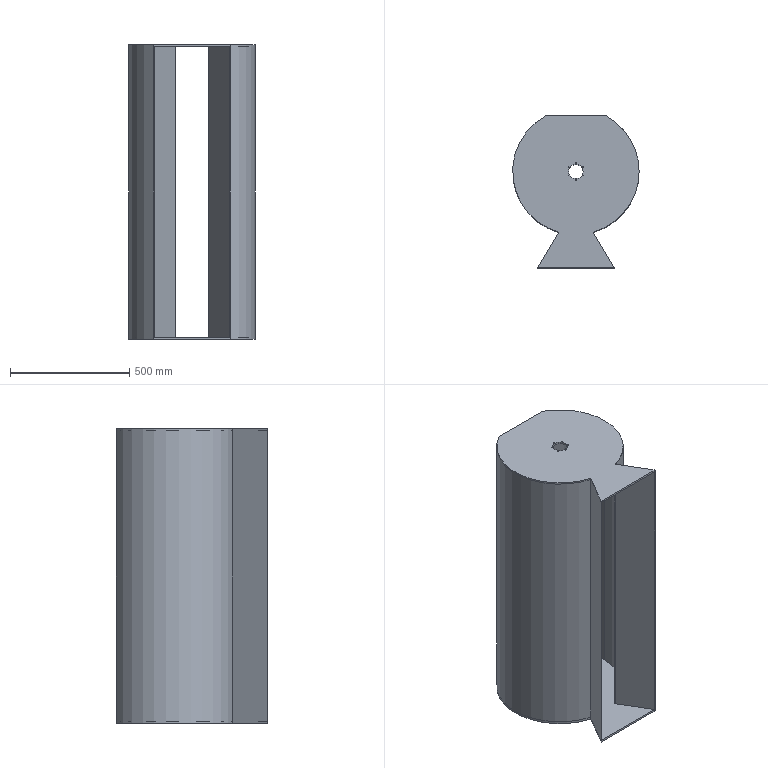Part | SolidWorks | features BaseBody 1 | 1 solid | 44 faces | box 530 x 635.026 x 1236 mm | volume 7825793 mm3 | cylinder 34 | plane 10 | commonest cylinder face diameters 2.703 x24 61 x4 526 x3 530 x3
STEP:
#1=CARTESIAN_POINT('',(30.5,0.,-610.));
#2=VERTEX_POINT('',#1);
#3=CARTESIAN_POINT('',(-30.5,0.,-610.));
#4=VERTEX_POINT('',#3);
#5=CARTESIAN_POINT('',(0.,0.,-610.));
#6=DIRECTION('',(0.,0.,-1.));
#7=DIRECTION('',(-1.,0.,0.));
#8=AXIS2_PLACEMENT_3D('',#5,#6,#7);
#9=CIRCLE('',#8,30.5);
#10=EDGE_CURVE('',#2,#4,#9,.T.);
#11=ORIENTED_EDGE('',*,*,#10,.F.);
#12=CARTESIAN_POINT('',(30.5,0.,-618.));
#13=VERTEX_POINT('',#12);
#14=CARTESIAN_POINT('',(30.5,0.,-610.));
#15=DIRECTION('',(0.,0.,-1.));
#16=VECTOR('',#15,1000.);
#17=LINE('',#14,#16);
#18=EDGE_CURVE('',#2,#13,#17,.T.);
#19=ORIENTED_EDGE('',*,*,#18,.T.);
#20=CARTESIAN_POINT('',(-30.5,0.,-618.));
#21=VERTEX_POINT('',#20);
#22=CARTESIAN_POINT('',(0.,0.,-618.));
#23=DIRECTION('',(0.,0.,-1.));
#24=DIRECTION('',(-1.,0.,0.));
#25=AXIS2_PLACEMENT_3D('',#22,#23,#24);
#26=CIRCLE('',#25,30.5);
#27=EDGE_CURVE('',#13,#21,#26,.T.);
#28=ORIENTED_EDGE('',*,*,#27,.T.);
#29=CARTESIAN_POINT('',(-30.5,0.,-610.));
#30=DIRECTION('',(0.,0.,-1.));
#31=VECTOR('',#30,1000.);
#32=LINE('',#29,#31);
#33=EDGE_CURVE('',#4,#21,#32,.T.);
#34=ORIENTED_EDGE('',*,*,#33,.F.);
#35=EDGE_LOOP('',(#11,#19,#28,#34));
#36=FACE_OUTER_BOUND('',#35,.T.);
#37=CARTESIAN_POINT('',(0.,0.,-610.));
#38=DIRECTION('',(0.,0.,-1.));
#39=DIRECTION('',(-1.,0.,0.));
#40=AXIS2_PLACEMENT_3D('',#37,#38,#39);
#41=CYLINDRICAL_SURFACE('',#40,30.5);
#42=ADVANCED_FACE('',(#36),#41,.F.);
#43=CARTESIAN_POINT('',(-29.105,17.584,-610.));
#44=VERTEX_POINT('',#43);
#45=CARTESIAN_POINT('',(-31.807,17.584,-610.));
#46=VERTEX_POINT('',#45);
#47=CARTESIAN_POINT('',(-30.456,17.584,-610.));
#48=DIRECTION('',(0.,0.,-1.));
#49=DIRECTION('',(-1.,0.,0.));
#50=AXIS2_PLACEMENT_3D('',#47,#48,#49);
#51=CIRCLE('',#50,1.351);
#52=EDGE_CURVE('',#44,#46,#51,.T.);
#53=ORIENTED_EDGE('',*,*,#52,.F.);
#54=CARTESIAN_POINT('',(-29.105,17.584,-618.));
#55=VERTEX_POINT('',#54);
#56=CARTESIAN_POINT('',(-29.105,17.584,618.));
#57=DIRECTION('',(0.,0.,-1.));
#58=VECTOR('',#57,1000.);
#59=LINE('',#56,#58);
#60=EDGE_CURVE('',#44,#55,#59,.T.);
#61=ORIENTED_EDGE('',*,*,#60,.T.);
#62=CARTESIAN_POINT('',(-31.807,17.584,-618.));
#63=VERTEX_POINT('',#62);
#64=CARTESIAN_POINT('',(-30.456,17.584,-618.));
#65=DIRECTION('',(0.,0.,-1.));
#66=DIRECTION('',(-1.,0.,0.));
#67=AXIS2_PLACEMENT_3D('',#64,#65,#66);
#68=CIRCLE('',#67,1.351);
#69=EDGE_CURVE('',#55,#63,#68,.T.);
#70=ORIENTED_EDGE('',*,*,#69,.T.);
#71=CARTESIAN_POINT('',(-31.807,17.584,618.));
#72=DIRECTION('',(0.,0.,-1.));
#73=VECTOR('',#72,1000.);
#74=LINE('',#71,#73);
#75=EDGE_CURVE('',#46,#63,#74,.T.);
#76=ORIENTED_EDGE('',*,*,#75,.F.);
#77=EDGE_LOOP('',(#53,#61,#70,#76));
#78=FACE_OUTER_BOUND('',#77,.T.);
#79=CARTESIAN_POINT('',(-30.456,17.584,618.));
#80=DIRECTION('',(0.,0.,-1.));
#81=DIRECTION('',(-1.,0.,0.));
#82=AXIS2_PLACEMENT_3D('',#79,#80,#81);
#83=CYLINDRICAL_SURFACE('',#82,1.351);
#84=ADVANCED_FACE('',(#78),#83,.F.);
#85=CARTESIAN_POINT('',(1.351,-35.168,-610.));
#86=VERTEX_POINT('',#85);
#87=CARTESIAN_POINT('',(-1.351,-35.168,-610.));
#88=VERTEX_POINT('',#87);
#89=CARTESIAN_POINT('',(0.,-35.168,-610.));
#90=DIRECTION('',(0.,0.,-1.));
#91=DIRECTION('',(-1.,0.,0.));
#92=AXIS2_PLACEMENT_3D('',#89,#90,#91);
#93=CIRCLE('',#92,1.351);
#94=EDGE_CURVE('',#86,#88,#93,.T.);
#95=ORIENTED_EDGE('',*,*,#94,.F.);
#96=CARTESIAN_POINT('',(1.351,-35.168,-618.));
#97=VERTEX_POINT('',#96);
#98=CARTESIAN_POINT('',(1.351,-35.168,618.));
#99=DIRECTION('',(0.,0.,-1.));
#100=VECTOR('',#99,1000.);
#101=LINE('',#98,#100);
#102=EDGE_CURVE('',#86,#97,#101,.T.);
#103=ORIENTED_EDGE('',*,*,#102,.T.);
#104=CARTESIAN_POINT('',(-1.351,-35.168,-618.));
#105=VERTEX_POINT('',#104);
#106=CARTESIAN_POINT('',(0.,-35.168,-618.));
#107=DIRECTION('',(0.,0.,-1.));
#108=DIRECTION('',(-1.,0.,0.));
#109=AXIS2_PLACEMENT_3D('',#106,#107,#108);
#110=CIRCLE('',#109,1.351);
#111=EDGE_CURVE('',#97,#105,#110,.T.);
#112=ORIENTED_EDGE('',*,*,#111,.T.);
#113=CARTESIAN_POINT('',(-1.351,-35.168,618.));
#114=DIRECTION('',(0.,0.,-1.));
#115=VECTOR('',#114,1000.);
#116=LINE('',#113,#115);
#117=EDGE_CURVE('',#88,#105,#116,.T.);
#118=ORIENTED_EDGE('',*,*,#117,.F.);
#119=EDGE_LOOP('',(#95,#103,#112,#118));
#120=FACE_OUTER_BOUND('',#119,.T.);
#121=CARTESIAN_POINT('',(0.,-35.168,618.));
#122=DIRECTION('',(0.,0.,-1.));
#123=DIRECTION('',(-1.,0.,0.));
#124=AXIS2_PLACEMENT_3D('',#121,#122,#123);
#125=CYLINDRICAL_SURFACE('',#124,1.351);
#126=ADVANCED_FACE('',(#120),#125,.F.);
#127=CARTESIAN_POINT('',(31.807,-17.584,-610.));
#128=VERTEX_POINT('',#127);
#129=CARTESIAN_POINT('',(29.105,-17.584,-610.));
#130=VERTEX_POINT('',#129);
#131=CARTESIAN_POINT('',(30.456,-17.584,-610.));
#132=DIRECTION('',(0.,0.,-1.));
#133=DIRECTION('',(-1.,0.,0.));
#134=AXIS2_PLACEMENT_3D('',#131,#132,#133);
#135=CIRCLE('',#134,1.351);
#136=EDGE_CURVE('',#128,#130,#135,.T.);
#137=ORIENTED_EDGE('',*,*,#136,.F.);
#138=CARTESIAN_POINT('',(31.807,-17.584,-618.));
#139=VERTEX_POINT('',#138);
#140=CARTESIAN_POINT('',(31.807,-17.584,618.));
#141=DIRECTION('',(0.,0.,-1.));
#142=VECTOR('',#141,1000.);
#143=LINE('',#140,#142);
#144=EDGE_CURVE('',#128,#139,#143,.T.);
#145=ORIENTED_EDGE('',*,*,#144,.T.);
#146=CARTESIAN_POINT('',(29.105,-17.584,-618.));
#147=VERTEX_POINT('',#146);
#148=CARTESIAN_POINT('',(30.456,-17.584,-618.));
#149=DIRECTION('',(0.,0.,-1.));
#150=DIRECTION('',(-1.,0.,0.));
#151=AXIS2_PLACEMENT_3D('',#148,#149,#150);
#152=CIRCLE('',#151,1.351);
#153=EDGE_CURVE('',#139,#147,#152,.T.);
#154=ORIENTED_EDGE('',*,*,#153,.T.);
#155=CARTESIAN_POINT('',(29.105,-17.584,618.));
#156=DIRECTION('',(0.,0.,-1.));
#157=VECTOR('',#156,1000.);
#158=LINE('',#155,#157);
#159=EDGE_CURVE('',#130,#147,#158,.T.);
#160=ORIENTED_EDGE('',*,*,#159,.F.);
#161=EDGE_LOOP('',(#137,#145,#154,#160));
#162=FACE_OUTER_BOUND('',#161,.T.);
#163=CARTESIAN_POINT('',(30.456,-17.584,618.));
#164=DIRECTION('',(0.,0.,-1.));
#165=DIRECTION('',(-1.,0.,0.));
#166=AXIS2_PLACEMENT_3D('',#163,#164,#165);
#167=CYLINDRICAL_SURFACE('',#166,1.351);
#168=ADVANCED_FACE('',(#162),#167,.F.);
#169=CARTESIAN_POINT('',(31.807,17.584,-610.));
#170=VERTEX_POINT('',#169);
#171=CARTESIAN_POINT('',(29.105,17.584,-610.));
#172=VERTEX_POINT('',#171);
#173=CARTESIAN_POINT('',(30.456,17.584,-610.));
#174=DIRECTION('',(0.,0.,-1.));
#175=DIRECTION('',(-1.,0.,0.));
#176=AXIS2_PLACEMENT_3D('',#173,#174,#175);
#177=CIRCLE('',#176,1.351);
#178=EDGE_CURVE('',#170,#172,#177,.T.);
#179=ORIENTED_EDGE('',*,*,#178,.F.);
#180=CARTESIAN_POINT('',(31.807,17.584,-618.));
#181=VERTEX_POINT('',#180);
#182=CARTESIAN_POINT('',(31.807,17.584,618.));
#183=DIRECTION('',(0.,0.,-1.));
#184=VECTOR('',#183,1000.);
#185=LINE('',#182,#184);
#186=EDGE_CURVE('',#170,#181,#185,.T.);
#187=ORIENTED_EDGE('',*,*,#186,.T.);
#188=CARTESIAN_POINT('',(29.105,17.584,-618.));
#189=VERTEX_POINT('',#188);
#190=CARTESIAN_POINT('',(30.456,17.584,-618.));
#191=DIRECTION('',(0.,0.,-1.));
#192=DIRECTION('',(-1.,0.,0.));
#193=AXIS2_PLACEMENT_3D('',#190,#191,#192);
#194=CIRCLE('',#193,1.351);
#195=EDGE_CURVE('',#181,#189,#194,.T.);
#196=ORIENTED_EDGE('',*,*,#195,.T.);
#197=CARTESIAN_POINT('',(29.105,17.584,618.));
#198=DIRECTION('',(0.,0.,-1.));
#199=VECTOR('',#198,1000.);
#200=LINE('',#197,#199);
#201=EDGE_CURVE('',#172,#189,#200,.T.);
#202=ORIENTED_EDGE('',*,*,#201,.F.);
#203=EDGE_LOOP('',(#179,#187,#196,#202));
#204=FACE_OUTER_BOUND('',#203,.T.);
#205=CARTESIAN_POINT('',(30.456,17.584,618.));
#206=DIRECTION('',(0.,0.,-1.));
#207=DIRECTION('',(-1.,0.,0.));
#208=AXIS2_PLACEMENT_3D('',#205,#206,#207);
#209=CYLINDRICAL_SURFACE('',#208,1.351);
#210=ADVANCED_FACE('',(#204),#209,.F.);
#211=CARTESIAN_POINT('',(1.351,35.168,-610.));
#212=VERTEX_POINT('',#211);
#213=CARTESIAN_POINT('',(-1.351,35.168,-610.));
#214=VERTEX_POINT('',#213);
#215=CARTESIAN_POINT('',(0.,35.168,-610.));
#216=DIRECTION('',(0.,0.,-1.));
#217=DIRECTION('',(-1.,0.,0.));
#218=AXIS2_PLACEMENT_3D('',#215,#216,#217);
#219=CIRCLE('',#218,1.351);
#220=EDGE_CURVE('',#212,#214,#219,.T.);
#221=ORIENTED_EDGE('',*,*,#220,.F.);
#222=CARTESIAN_POINT('',(1.351,35.168,-618.));
#223=VERTEX_POINT('',#222);
#224=CARTESIAN_POINT('',(1.351,35.168,618.));
#225=DIRECTION('',(0.,0.,-1.));
#226=VECTOR('',#225,1000.);
#227=LINE('',#224,#226);
#228=EDGE_CURVE('',#212,#223,#227,.T.);
#229=ORIENTED_EDGE('',*,*,#228,.T.);
#230=CARTESIAN_POINT('',(-1.351,35.168,-618.));
#231=VERTEX_POINT('',#230);
#232=CARTESIAN_POINT('',(0.,35.168,-618.));
#233=DIRECTION('',(0.,0.,-1.));
#234=DIRECTION('',(-1.,0.,0.));
#235=AXIS2_PLACEMENT_3D('',#232,#233,#234);
#236=CIRCLE('',#235,1.351);
#237=EDGE_CURVE('',#223,#231,#236,.T.);
#238=ORIENTED_EDGE('',*,*,#237,.T.);
#239=CARTESIAN_POINT('',(-1.351,35.168,618.));
#240=DIRECTION('',(0.,0.,-1.));
#241=VECTOR('',#240,1000.);
#242=LINE('',#239,#241);
#243=EDGE_CURVE('',#214,#231,#242,.T.);
#244=ORIENTED_EDGE('',*,*,#243,.F.);
#245=EDGE_LOOP('',(#221,#229,#238,#244));
#246=FACE_OUTER_BOUND('',#245,.T.);
#247=CARTESIAN_POINT('',(0.,35.168,618.));
#248=DIRECTION('',(0.,0.,-1.));
#249=DIRECTION('',(-1.,0.,0.));
#250=AXIS2_PLACEMENT_3D('',#247,#248,#249);
#251=CYLINDRICAL_SURFACE('',#250,1.351);
#252=ADVANCED_FACE('',(#246),#251,.F.);
#253=CARTESIAN_POINT('',(-29.105,-17.584,-610.));
#254=VERTEX_POINT('',#253);
#255=CARTESIAN_POINT('',(-31.807,-17.584,-610.));
#256=VERTEX_POINT('',#255);
#257=CARTESIAN_POINT('',(-30.456,-17.584,-610.));
#258=DIRECTION('',(0.,0.,-1.));
#259=DIRECTION('',(-1.,0.,0.));
#260=AXIS2_PLACEMENT_3D('',#257,#258,#259);
#261=CIRCLE('',#260,1.351);
#262=EDGE_CURVE('',#254,#256,#261,.T.);
#263=ORIENTED_EDGE('',*,*,#262,.F.);
#264=CARTESIAN_POINT('',(-29.105,-17.584,-618.));
#265=VERTEX_POINT('',#264);
#266=CARTESIAN_POINT('',(-29.105,-17.584,618.));
#267=DIRECTION('',(0.,0.,-1.));
#268=VECTOR('',#267,1000.);
#269=LINE('',#266,#268);
#270=EDGE_CURVE('',#254,#265,#269,.T.);
#271=ORIENTED_EDGE('',*,*,#270,.T.);
#272=CARTESIAN_POINT('',(-31.807,-17.584,-618.));
#273=VERTEX_POINT('',#272);
#274=CARTESIAN_POINT('',(-30.456,-17.584,-618.));
#275=DIRECTION('',(0.,0.,-1.));
#276=DIRECTION('',(-1.,0.,0.));
#277=AXIS2_PLACEMENT_3D('',#274,#275,#276);
#278=CIRCLE('',#277,1.351);
#279=EDGE_CURVE('',#265,#273,#278,.T.);
#280=ORIENTED_EDGE('',*,*,#279,.T.);
#281=CARTESIAN_POINT('',(-31.807,-17.584,618.));
#282=DIRECTION('',(0.,0.,-1.));
#283=VECTOR('',#282,1000.);
#284=LINE('',#281,#283);
#285=EDGE_CURVE('',#256,#273,#284,.T.);
#286=ORIENTED_EDGE('',*,*,#285,.F.);
#287=EDGE_LOOP('',(#263,#271,#280,#286));
#288=FACE_OUTER_BOUND('',#287,.T.);
#289=CARTESIAN_POINT('',(-30.456,-17.584,618.));
#290=DIRECTION('',(0.,0.,-1.));
#291=DIRECTION('',(-1.,0.,0.));
#292=AXIS2_PLACEMENT_3D('',#289,#290,#291);
#293=CYLINDRICAL_SURFACE('',#292,1.351);
#294=ADVANCED_FACE('',(#288),#293,.F.);
#295=CARTESIAN_POINT('',(72.49,-254.892,-618.));
#296=VERTEX_POINT('',#295);
#297=CARTESIAN_POINT('',(265.,0.,-618.));
#298=VERTEX_POINT('',#297);
#299=CARTESIAN_POINT('',(0.,0.,-618.));
#300=DIRECTION('',(0.,0.,1.));
#301=DIRECTION('',(1.,0.,0.));
#302=AXIS2_PLACEMENT_3D('',#299,#300,#301);
#303=CIRCLE('',#302,265.);
#304=EDGE_CURVE('',#296,#298,#303,.T.);
#305=ORIENTED_EDGE('',*,*,#304,.T.);
#306=CARTESIAN_POINT('',(265.,0.,618.));
#307=VERTEX_POINT('',#306);
#308=CARTESIAN_POINT('',(265.,0.,0.));
#309=DIRECTION('',(0.,0.,1.));
#310=VECTOR('',#309,1000.);
#311=LINE('',#308,#310);
#312=EDGE_CURVE('',#298,#307,#311,.T.);
#313=ORIENTED_EDGE('',*,*,#312,.T.);
#314=CARTESIAN_POINT('',(72.49,-254.892,618.));
#315=VERTEX_POINT('',#314);
#316=CARTESIAN_POINT('',(0.,0.,618.));
#317=DIRECTION('',(0.,0.,1.));
#318=DIRECTION('',(1.,0.,0.));
#319=AXIS2_PLACEMENT_3D('',#316,#317,#318);
#320=CIRCLE('',#319,265.);
#321=EDGE_CURVE('',#315,#307,#320,.T.);
#322=ORIENTED_EDGE('',*,*,#321,.F.);
#323=CARTESIAN_POINT('',(72.49,-254.892,0.));
#324=DIRECTION('',(0.,0.,-1.));
#325=VECTOR('',#324,1000.);
#326=LINE('',#323,#325);
#327=EDGE_CURVE('',#315,#296,#326,.T.);
#328=ORIENTED_EDGE('',*,*,#327,.T.);
#329=EDGE_LOOP('',(#305,#313,#322,#328));
#330=FACE_OUTER_BOUND('',#329,.T.);
#331=CARTESIAN_POINT('',(0.,0.,0.));
#332=DIRECTION('',(0.,0.,1.));
#333=DIRECTION('',(1.,0.,0.));
#334=AXIS2_PLACEMENT_3D('',#331,#332,#333);
#335=CYLINDRICAL_SURFACE('',#334,265.);
#336=ADVANCED_FACE('',(#330),#335,.T.);
#337=CARTESIAN_POINT('',(263.,0.,-610.));
#338=VERTEX_POINT('',#337);
#339=CARTESIAN_POINT('',(124.086,231.887,-610.));
#340=VERTEX_POINT('',#339);
#341=CARTESIAN_POINT('',(0.,0.,-610.));
#342=DIRECTION('',(0.,0.,1.));
#343=DIRECTION('',(1.,0.,0.));
#344=AXIS2_PLACEMENT_3D('',#341,#342,#343);
#345=CIRCLE('',#344,263.);
#346=EDGE_CURVE('',#338,#340,#345,.T.);
#347=ORIENTED_EDGE('',*,*,#346,.F.);
#348=CARTESIAN_POINT('',(263.,0.,610.));
#349=VERTEX_POINT('',#348);
#350=CARTESIAN_POINT('',(263.,0.,0.));
#351=DIRECTION('',(0.,0.,1.));
#352=VECTOR('',#351,1000.);
#353=LINE('',#350,#352);
#354=EDGE_CURVE('',#338,#349,#353,.T.);
#355=ORIENTED_EDGE('',*,*,#354,.T.);
#356=CARTESIAN_POINT('',(124.086,231.887,610.));
#357=VERTEX_POINT('',#356);
#358=CARTESIAN_POINT('',(0.,0.,610.));
#359=DIRECTION('',(0.,0.,-1.));
#360=DIRECTION('',(1.,0.,0.));
#361=AXIS2_PLACEMENT_3D('',#358,#359,#360);
#362=CIRCLE('',#361,263.);
#363=EDGE_CURVE('',#357,#349,#362,.T.);
#364=ORIENTED_EDGE('',*,*,#363,.F.);
#365=CARTESIAN_POINT('',(124.086,231.887,0.));
#366=DIRECTION('',(0.,0.,1.));
#367=VECTOR('',#366,1000.);
#368=LINE('',#365,#367);
#369=EDGE_CURVE('',#340,#357,#368,.T.);
#370=ORIENTED_EDGE('',*,*,#369,.F.);
#371=EDGE_LOOP('',(#347,#355,#364,#370));
#372=FACE_OUTER_BOUND('',#371,.T.);
#373=CARTESIAN_POINT('',(0.,0.,0.));
#374=DIRECTION('',(0.,0.,1.));
#375=DIRECTION('',(1.,0.,0.));
#376=AXIS2_PLACEMENT_3D('',#373,#374,#375);
#377=CYLINDRICAL_SURFACE('',#376,263.);
#378=ADVANCED_FACE('',(#372),#377,.F.);
#379=CARTESIAN_POINT('',(30.5,0.,618.));
#380=VERTEX_POINT('',#379);
#381=CARTESIAN_POINT('',(-30.5,0.,618.));
#382=VERTEX_POINT('',#381);
#383=CARTESIAN_POINT('',(0.,0.,618.));
#384=DIRECTION('',(0.,0.,-1.));
#385=DIRECTION('',(-1.,0.,0.));
#386=AXIS2_PLACEMENT_3D('',#383,#384,#385);
#387=CIRCLE('',#386,30.5);
#388=EDGE_CURVE('',#380,#382,#387,.T.);
#389=ORIENTED_EDGE('',*,*,#388,.F.);
#390=CARTESIAN_POINT('',(30.5,0.,610.));
#391=VERTEX_POINT('',#390);
#392=CARTESIAN_POINT('',(30.5,0.,610.));
#393=DIRECTION('',(0.,0.,-1.));
#394=VECTOR('',#393,1000.);
#395=LINE('',#392,#394);
#396=EDGE_CURVE('',#380,#391,#395,.T.);
#397=ORIENTED_EDGE('',*,*,#396,.T.);
#398=CARTESIAN_POINT('',(-30.5,0.,610.));
#399=VERTEX_POINT('',#398);
#400=CARTESIAN_POINT('',(0.,0.,610.));
#401=DIRECTION('',(0.,0.,1.));
#402=DIRECTION('',(-1.,0.,0.));
#403=AXIS2_PLACEMENT_3D('',#400,#401,#402);
#404=CIRCLE('',#403,30.5);
#405=EDGE_CURVE('',#399,#391,#404,.T.);
#406=ORIENTED_EDGE('',*,*,#405,.F.);
#407=CARTESIAN_POINT('',(-30.5,0.,610.));
#408=DIRECTION('',(0.,0.,-1.));
#409=VECTOR('',#408,1000.);
#410=LINE('',#407,#409);
#411=EDGE_CURVE('',#382,#399,#410,.T.);
#412=ORIENTED_EDGE('',*,*,#411,.F.);
#413=EDGE_LOOP('',(#389,#397,#406,#412));
#414=FACE_OUTER_BOUND('',#413,.T.);
#415=CARTESIAN_POINT('',(0.,0.,610.));
#416=DIRECTION('',(0.,0.,-1.));
#417=DIRECTION('',(-1.,0.,0.));
#418=AXIS2_PLACEMENT_3D('',#415,#416,#417);
#419=CYLINDRICAL_SURFACE('',#418,30.5);
#420=ADVANCED_FACE('',(#414),#419,.F.);
#421=CARTESIAN_POINT('',(-29.105,17.584,618.));
#422=VERTEX_POINT('',#421);
#423=CARTESIAN_POINT('',(-31.807,17.584,618.));
#424=VERTEX_POINT('',#423);
#425=CARTESIAN_POINT('',(-30.456,17.584,618.));
#426=DIRECTION('',(0.,0.,-1.));
#427=DIRECTION('',(-1.,0.,0.));
#428=AXIS2_PLACEMENT_3D('',#425,#426,#427);
#429=CIRCLE('',#428,1.351);
#430=EDGE_CURVE('',#422,#424,#429,.T.);
#431=ORIENTED_EDGE('',*,*,#430,.F.);
#432=CARTESIAN_POINT('',(-29.105,17.584,610.));
#433=VERTEX_POINT('',#432);
#434=CARTESIAN_POINT('',(-29.105,17.584,618.));
#435=DIRECTION('',(0.,0.,-1.));
#436=VECTOR('',#435,1000.);
#437=LINE('',#434,#436);
#438=EDGE_CURVE('',#422,#433,#437,.T.);
#439=ORIENTED_EDGE('',*,*,#438,.T.);
#440=CARTESIAN_POINT('',(-31.807,17.584,610.));
#441=VERTEX_POINT('',#440);
#442=CARTESIAN_POINT('',(-30.456,17.584,610.));
#443=DIRECTION('',(0.,0.,1.));
#444=DIRECTION('',(-1.,0.,0.));
#445=AXIS2_PLACEMENT_3D('',#442,#443,#444);
#446=CIRCLE('',#445,1.351);
#447=EDGE_CURVE('',#441,#433,#446,.T.);
#448=ORIENTED_EDGE('',*,*,#447,.F.);
#449=CARTESIAN_POINT('',(-31.807,17.584,618.));
#450=DIRECTION('',(0.,0.,-1.));
#451=VECTOR('',#450,1000.);
#452=LINE('',#449,#451);
#453=EDGE_CURVE('',#424,#441,#452,.T.);
#454=ORIENTED_EDGE('',*,*,#453,.F.);
#455=EDGE_LOOP('',(#431,#439,#448,#454));
#456=FACE_OUTER_BOUND('',#455,.T.);
#457=CARTESIAN_POINT('',(-30.456,17.584,618.));
#458=DIRECTION('',(0.,0.,-1.));
#459=DIRECTION('',(-1.,0.,0.));
#460=AXIS2_PLACEMENT_3D('',#457,#458,#459);
#461=CYLINDRICAL_SURFACE('',#460,1.351);
#462=ADVANCED_FACE('',(#456),#461,.F.);
#463=CARTESIAN_POINT('',(1.351,-35.168,618.));
#464=VERTEX_POINT('',#463);
#465=CARTESIAN_POINT('',(-1.351,-35.168,618.));
#466=VERTEX_POINT('',#465);
#467=CARTESIAN_POINT('',(0.,-35.168,618.));
#468=DIRECTION('',(0.,0.,-1.));
#469=DIRECTION('',(-1.,0.,0.));
#470=AXIS2_PLACEMENT_3D('',#467,#468,#469);
#471=CIRCLE('',#470,1.351);
#472=EDGE_CURVE('',#464,#466,#471,.T.);
#473=ORIENTED_EDGE('',*,*,#472,.F.);
#474=CARTESIAN_POINT('',(1.351,-35.168,610.));
#475=VERTEX_POINT('',#474);
#476=CARTESIAN_POINT('',(1.351,-35.168,618.));
#477=DIRECTION('',(0.,0.,-1.));
#478=VECTOR('',#477,1000.);
#479=LINE('',#476,#478);
#480=EDGE_CURVE('',#464,#475,#479,.T.);
#481=ORIENTED_EDGE('',*,*,#480,.T.);
#482=CARTESIAN_POINT('',(-1.351,-35.168,610.));
#483=VERTEX_POINT('',#482);
#484=CARTESIAN_POINT('',(0.,-35.168,610.));
#485=DIRECTION('',(0.,0.,1.));
#486=DIRECTION('',(-1.,0.,0.));
#487=AXIS2_PLACEMENT_3D('',#484,#485,#486);
#488=CIRCLE('',#487,1.351);
#489=EDGE_CURVE('',#483,#475,#488,.T.);
#490=ORIENTED_EDGE('',*,*,#489,.F.);
#491=CARTESIAN_POINT('',(-1.351,-35.168,618.));
#492=DIRECTION('',(0.,0.,-1.));
#493=VECTOR('',#492,1000.);
#494=LINE('',#491,#493);
#495=EDGE_CURVE('',#466,#483,#494,.T.);
#496=ORIENTED_EDGE('',*,*,#495,.F.);
#497=EDGE_LOOP('',(#473,#481,#490,#496));
#498=FACE_OUTER_BOUND('',#497,.T.);
#499=CARTESIAN_POINT('',(0.,-35.168,618.));
#500=DIRECTION('',(0.,0.,-1.));
#501=DIRECTION('',(-1.,0.,0.));
#502=AXIS2_PLACEMENT_3D('',#499,#500,#501);
#503=CYLINDRICAL_SURFACE('',#502,1.351);
#504=ADVANCED_FACE('',(#498),#503,.F.);
#505=CARTESIAN_POINT('',(31.807,-17.584,618.));
#506=VERTEX_POINT('',#505);
#507=CARTESIAN_POINT('',(29.105,-17.584,618.));
#508=VERTEX_POINT('',#507);
#509=CARTESIAN_POINT('',(30.456,-17.584,618.));
#510=DIRECTION('',(0.,0.,-1.));
#511=DIRECTION('',(-1.,0.,0.));
#512=AXIS2_PLACEMENT_3D('',#509,#510,#511);
#513=CIRCLE('',#512,1.351);
#514=EDGE_CURVE('',#506,#508,#513,.T.);
#515=ORIENTED_EDGE('',*,*,#514,.F.);
#516=CARTESIAN_POINT('',(31.807,-17.584,610.));
#517=VERTEX_POINT('',#516);
#518=CARTESIAN_POINT('',(31.807,-17.584,618.));
#519=DIRECTION('',(0.,0.,-1.));
#520=VECTOR('',#519,1000.);
#521=LINE('',#518,#520);
#522=EDGE_CURVE('',#506,#517,#521,.T.);
#523=ORIENTED_EDGE('',*,*,#522,.T.);
#524=CARTESIAN_POINT('',(29.105,-17.584,610.));
#525=VERTEX_POINT('',#524);
#526=CARTESIAN_POINT('',(30.456,-17.584,610.));
#527=DIRECTION('',(0.,0.,1.));
#528=DIRECTION('',(-1.,0.,0.));
#529=AXIS2_PLACEMENT_3D('',#526,#527,#528);
#530=CIRCLE('',#529,1.351);
#531=EDGE_CURVE('',#525,#517,#530,.T.);
#532=ORIENTED_EDGE('',*,*,#531,.F.);
#533=CARTESIAN_POINT('',(29.105,-17.584,618.));
#534=DIRECTION('',(0.,0.,-1.));
#535=VECTOR('',#534,1000.);
#536=LINE('',#533,#535);
#537=EDGE_CURVE('',#508,#525,#536,.T.);
#538=ORIENTED_EDGE('',*,*,#537,.F.);
#539=EDGE_LOOP('',(#515,#523,#532,#538));
#540=FACE_OUTER_BOUND('',#539,.T.);
#541=CARTESIAN_POINT('',(30.456,-17.584,618.));
#542=DIRECTION('',(0.,0.,-1.));
#543=DIRECTION('',(-1.,0.,0.));
#544=AXIS2_PLACEMENT_3D('',#541,#542,#543);
#545=CYLINDRICAL_SURFACE('',#544,1.351);
#546=ADVANCED_FACE('',(#540),#545,.F.);
#547=CARTESIAN_POINT('',(31.807,17.584,618.));
#548=VERTEX_POINT('',#547);
#549=CARTESIAN_POINT('',(29.105,17.584,618.));
#550=VERTEX_POINT('',#549);
#551=CARTESIAN_POINT('',(30.456,17.584,618.));
#552=DIRECTION('',(0.,0.,-1.));
#553=DIRECTION('',(-1.,0.,0.));
#554=AXIS2_PLACEMENT_3D('',#551,#552,#553);
#555=CIRCLE('',#554,1.351);
#556=EDGE_CURVE('',#548,#550,#555,.T.);
#557=ORIENTED_EDGE('',*,*,#556,.F.);
#558=CARTESIAN_POINT('',(31.807,17.584,610.));
#559=VERTEX_POINT('',#558);
#560=CARTESIAN_POINT('',(31.807,17.584,618.));
#561=DIRECTION('',(0.,0.,-1.));
#562=VECTOR('',#561,1000.);
#563=LINE('',#560,#562);
#564=EDGE_CURVE('',#548,#559,#563,.T.);
#565=ORIENTED_EDGE('',*,*,#564,.T.);
#566=CARTESIAN_POINT('',(29.105,17.584,610.));
#567=VERTEX_POINT('',#566);
#568=CARTESIAN_POINT('',(30.456,17.584,610.));
#569=DIRECTION('',(0.,0.,1.));
#570=DIRECTION('',(-1.,0.,0.));
#571=AXIS2_PLACEMENT_3D('',#568,#569,#570);
#572=CIRCLE('',#571,1.351);
#573=EDGE_CURVE('',#567,#559,#572,.T.);
#574=ORIENTED_EDGE('',*,*,#573,.F.);
#575=CARTESIAN_POINT('',(29.105,17.584,618.));
#576=DIRECTION('',(0.,0.,-1.));
#577=VECTOR('',#576,1000.);
#578=LINE('',#575,#577);
#579=EDGE_CURVE('',#550,#567,#578,.T.);
#580=ORIENTED_EDGE('',*,*,#579,.F.);
#581=EDGE_LOOP('',(#557,#565,#574,#580));
#582=FACE_OUTER_BOUND('',#581,.T.);
#583=CARTESIAN_POINT('',(30.456,17.584,618.));
#584=DIRECTION('',(0.,0.,-1.));
#585=DIRECTION('',(-1.,0.,0.));
#586=AXIS2_PLACEMENT_3D('',#583,#584,#585);
#587=CYLINDRICAL_SURFACE('',#586,1.351);
#588=ADVANCED_FACE('',(#582),#587,.F.);
#589=CARTESIAN_POINT('',(1.351,35.168,618.));
#590=VERTEX_POINT('',#589);
#591=CARTESIAN_POINT('',(-1.351,35.168,618.));
#592=VERTEX_POINT('',#591);
#593=CARTESIAN_POINT('',(0.,35.168,618.));
#594=DIRECTION('',(0.,0.,-1.));
#595=DIRECTION('',(-1.,0.,0.));
#596=AXIS2_PLACEMENT_3D('',#593,#594,#595);
#597=CIRCLE('',#596,1.351);
#598=EDGE_CURVE('',#590,#592,#597,.T.);
#599=ORIENTED_EDGE('',*,*,#598,.F.);
#600=CARTESIAN_POINT('',(1.351,35.168,610.));
#601=VERTEX_POINT('',#600);
#602=CARTESIAN_POINT('',(1.351,35.168,618.));
#603=DIRECTION('',(0.,0.,-1.));
#604=VECTOR('',#603,1000.);
#605=LINE('',#602,#604);
#606=EDGE_CURVE('',#590,#601,#605,.T.);
#607=ORIENTED_EDGE('',*,*,#606,.T.);
#608=CARTESIAN_POINT('',(-1.351,35.168,610.));
#609=VERTEX_POINT('',#608);
#610=CARTESIAN_POINT('',(0.,35.168,610.));
#611=DIRECTION('',(0.,0.,1.));
#612=DIRECTION('',(-1.,0.,0.));
#613=AXIS2_PLACEMENT_3D('',#610,#611,#612);
#614=CIRCLE('',#613,1.351);
#615=EDGE_CURVE('',#609,#601,#614,.T.);
#616=ORIENTED_EDGE('',*,*,#615,.F.);
#617=CARTESIAN_POINT('',(-1.351,35.168,618.));
#618=DIRECTION('',(0.,0.,-1.));
#619=VECTOR('',#618,1000.);
#620=LINE('',#617,#619);
#621=EDGE_CURVE('',#592,#609,#620,.T.);
#622=ORIENTED_EDGE('',*,*,#621,.F.);
#623=EDGE_LOOP('',(#599,#607,#616,#622));
#624=FACE_OUTER_BOUND('',#623,.T.);
#625=CARTESIAN_POINT('',(0.,35.168,618.));
#626=DIRECTION('',(0.,0.,-1.));
#627=DIRECTION('',(-1.,0.,0.));
#628=AXIS2_PLACEMENT_3D('',#625,#626,#627);
#629=CYLINDRICAL_SURFACE('',#628,1.351);
#630=ADVANCED_FACE('',(#624),#629,.F.);
#631=CARTESIAN_POINT('',(-29.105,-17.584,618.));
#632=VERTEX_POINT('',#631);
#633=CARTESIAN_POINT('',(-31.807,-17.584,618.));
#634=VERTEX_POINT('',#633);
#635=CARTESIAN_POINT('',(-30.456,-17.584,618.));
#636=DIRECTION('',(0.,0.,-1.));
#637=DIRECTION('',(-1.,0.,0.));
#638=AXIS2_PLACEMENT_3D('',#635,#636,#637);
#639=CIRCLE('',#638,1.351);
#640=EDGE_CURVE('',#632,#634,#639,.T.);
#641=ORIENTED_EDGE('',*,*,#640,.F.);
#642=CARTESIAN_POINT('',(-29.105,-17.584,610.));
#643=VERTEX_POINT('',#642);
#644=CARTESIAN_POINT('',(-29.105,-17.584,618.));
#645=DIRECTION('',(0.,0.,-1.));
#646=VECTOR('',#645,1000.);
#647=LINE('',#644,#646);
#648=EDGE_CURVE('',#632,#643,#647,.T.);
#649=ORIENTED_EDGE('',*,*,#648,.T.);
#650=CARTESIAN_POINT('',(-31.807,-17.584,610.));
#651=VERTEX_POINT('',#650);
#652=CARTESIAN_POINT('',(-30.456,-17.584,610.));
#653=DIRECTION('',(0.,0.,1.));
#654=DIRECTION('',(-1.,0.,0.));
#655=AXIS2_PLACEMENT_3D('',#652,#653,#654);
#656=CIRCLE('',#655,1.351);
#657=EDGE_CURVE('',#651,#643,#656,.T.);
#658=ORIENTED_EDGE('',*,*,#657,.F.);
#659=CARTESIAN_POINT('',(-31.807,-17.584,618.));
#660=DIRECTION('',(0.,0.,-1.));
#661=VECTOR('',#660,1000.);
#662=LINE('',#659,#661);
#663=EDGE_CURVE('',#634,#651,#662,.T.);
#664=ORIENTED_EDGE('',*,*,#663,.F.);
#665=EDGE_LOOP('',(#641,#649,#658,#664));
#666=FACE_OUTER_BOUND('',#665,.T.);
#667=CARTESIAN_POINT('',(-30.456,-17.584,618.));
#668=DIRECTION('',(0.,0.,-1.));
#669=DIRECTION('',(-1.,0.,0.));
#670=AXIS2_PLACEMENT_3D('',#667,#668,#669);
#671=CYLINDRICAL_SURFACE('',#670,1.351);
#672=ADVANCED_FACE('',(#666),#671,.F.);
#673=CARTESIAN_POINT('',(-128.27,231.887,618.));
#674=VERTEX_POINT('',#673);
#675=CARTESIAN_POINT('',(-128.27,231.887,-618.));
#676=VERTEX_POINT('',#675);
#677=CARTESIAN_POINT('',(-128.27,231.887,0.));
#678=DIRECTION('',(0.,0.,-1.));
#679=VECTOR('',#678,1000.);
#680=LINE('',#677,#679);
#681=EDGE_CURVE('',#674,#676,#680,.T.);
#682=ORIENTED_EDGE('',*,*,#681,.T.);
#683=CARTESIAN_POINT('',(-72.045,-255.019,-618.));
#684=VERTEX_POINT('',#683);
#685=CARTESIAN_POINT('',(0.,0.,-618.));
#686=DIRECTION('',(0.,0.,1.));
#687=DIRECTION('',(1.,0.,0.));
#688=AXIS2_PLACEMENT_3D('',#685,#686,#687);
#689=CIRCLE('',#688,265.);
#690=EDGE_CURVE('',#676,#684,#689,.T.);
#691=ORIENTED_EDGE('',*,*,#690,.T.);
#692=CARTESIAN_POINT('',(-72.045,-255.019,618.));
#693=VERTEX_POINT('',#692);
#694=CARTESIAN_POINT('',(-72.045,-255.019,0.));
#695=DIRECTION('',(0.,0.,1.));
#696=VECTOR('',#695,1000.);
#697=LINE('',#694,#696);
#698=EDGE_CURVE('',#684,#693,#697,.T.);
#699=ORIENTED_EDGE('',*,*,#698,.T.);
#700=CARTESIAN_POINT('',(0.,0.,618.));
#701=DIRECTION('',(0.,0.,-1.));
#702=DIRECTION('',(1.,0.,0.));
#703=AXIS2_PLACEMENT_3D('',#700,#701,#702);
#704=CIRCLE('',#703,265.);
#705=EDGE_CURVE('',#693,#674,#704,.T.);
#706=ORIENTED_EDGE('',*,*,#705,.T.);
#707=EDGE_LOOP('',(#682,#691,#699,#706));
#708=FACE_OUTER_BOUND('',#707,.T.);
#709=CARTESIAN_POINT('',(0.,0.,0.));
#710=DIRECTION('',(0.,0.,1.));
#711=DIRECTION('',(1.,0.,0.));
#712=AXIS2_PLACEMENT_3D('',#709,#710,#711);
#713=CYLINDRICAL_SURFACE('',#712,265.);
#714=ADVANCED_FACE('',(#708),#713,.T.);
#715=CARTESIAN_POINT('',(0.,0.,-618.));
#716=DIRECTION('',(0.,0.,-1.));
#717=DIRECTION('',(-1.,0.,0.));
#718=AXIS2_PLACEMENT_3D('',#715,#716,#717);
#719=CIRCLE('',#718,30.5);
#720=EDGE_CURVE('',#21,#13,#719,.T.);
#721=ORIENTED_EDGE('',*,*,#720,.F.);
#722=ORIENTED_EDGE('',*,*,#27,.F.);
#723=EDGE_LOOP('',(#721,#722));
#724=FACE_BOUND('',#723,.T.);
#725=CARTESIAN_POINT('',(-30.456,17.584,-618.));
#726=DIRECTION('',(0.,0.,-1.));
#727=DIRECTION('',(-1.,0.,0.));
#728=AXIS2_PLACEMENT_3D('',#725,#726,#727);
#729=CIRCLE('',#728,1.351);
#730=EDGE_CURVE('',#63,#55,#729,.T.);
#731=ORIENTED_EDGE('',*,*,#730,.F.);
#732=ORIENTED_EDGE('',*,*,#69,.F.);
#733=EDGE_LOOP('',(#731,#732));
#734=FACE_BOUND('',#733,.T.);
#735=CARTESIAN_POINT('',(0.,-35.168,-618.));
#736=DIRECTION('',(0.,0.,-1.));
#737=DIRECTION('',(-1.,0.,0.));
#738=AXIS2_PLACEMENT_3D('',#735,#736,#737);
#739=CIRCLE('',#738,1.351);
#740=EDGE_CURVE('',#105,#97,#739,.T.);
#741=ORIENTED_EDGE('',*,*,#740,.F.);
#742=ORIENTED_EDGE('',*,*,#111,.F.);
#743=EDGE_LOOP('',(#741,#742));
#744=FACE_BOUND('',#743,.T.);
#745=CARTESIAN_POINT('',(30.456,-17.584,-618.));
#746=DIRECTION('',(0.,0.,-1.));
#747=DIRECTION('',(-1.,0.,0.));
#748=AXIS2_PLACEMENT_3D('',#745,#746,#747);
#749=CIRCLE('',#748,1.351);
#750=EDGE_CURVE('',#147,#139,#749,.T.);
#751=ORIENTED_EDGE('',*,*,#750,.F.);
#752=ORIENTED_EDGE('',*,*,#153,.F.);
#753=EDGE_LOOP('',(#751,#752));
#754=FACE_BOUND('',#753,.T.);
#755=CARTESIAN_POINT('',(30.456,17.584,-618.));
#756=DIRECTION('',(0.,0.,-1.));
#757=DIRECTION('',(-1.,0.,0.));
#758=AXIS2_PLACEMENT_3D('',#755,#756,#757);
#759=CIRCLE('',#758,1.351);
#760=EDGE_CURVE('',#189,#181,#759,.T.);
#761=ORIENTED_EDGE('',*,*,#760,.F.);
#762=ORIENTED_EDGE('',*,*,#195,.F.);
#763=EDGE_LOOP('',(#761,#762));
#764=FACE_BOUND('',#763,.T.);
#765=CARTESIAN_POINT('',(0.,35.168,-618.));
#766=DIRECTION('',(0.,0.,-1.));
#767=DIRECTION('',(-1.,0.,0.));
#768=AXIS2_PLACEMENT_3D('',#765,#766,#767);
#769=CIRCLE('',#768,1.351);
#770=EDGE_CURVE('',#231,#223,#769,.T.);
#771=ORIENTED_EDGE('',*,*,#770,.F.);
#772=ORIENTED_EDGE('',*,*,#237,.F.);
#773=EDGE_LOOP('',(#771,#772));
#774=FACE_BOUND('',#773,.T.);
#775=CARTESIAN_POINT('',(-30.456,-17.584,-618.));
#776=DIRECTION('',(0.,0.,-1.));
#777=DIRECTION('',(-1.,0.,0.));
#778=AXIS2_PLACEMENT_3D('',#775,#776,#777);
#779=CIRCLE('',#778,1.351);
#780=EDGE_CURVE('',#273,#265,#779,.T.);
#781=ORIENTED_EDGE('',*,*,#780,.F.);
#782=ORIENTED_EDGE('',*,*,#279,.F.);
#783=EDGE_LOOP('',(#781,#782));
#784=FACE_BOUND('',#783,.T.);
#785=ORIENTED_EDGE('',*,*,#690,.F.);
#786=CARTESIAN_POINT('',(128.27,231.887,-618.));
#787=VERTEX_POINT('',#786);
#788=CARTESIAN_POINT('',(0.,231.887,-618.));
#789=DIRECTION('',(-1.,0.,0.));
#790=VECTOR('',#789,1000.);
#791=LINE('',#788,#790);
#792=EDGE_CURVE('',#787,#676,#791,.T.);
#793=ORIENTED_EDGE('',*,*,#792,.F.);
#794=CARTESIAN_POINT('',(0.,0.,-618.));
#795=DIRECTION('',(0.,0.,1.));
#796=DIRECTION('',(1.,0.,0.));
#797=AXIS2_PLACEMENT_3D('',#794,#795,#796);
#798=CIRCLE('',#797,265.);
#799=EDGE_CURVE('',#298,#787,#798,.T.);
#800=ORIENTED_EDGE('',*,*,#799,.F.);
#801=ORIENTED_EDGE('',*,*,#304,.F.);
#802=CARTESIAN_POINT('',(160.281,-403.139,-618.));
#803=VERTEX_POINT('',#802);
#804=CARTESIAN_POINT('',(160.281,-403.139,-618.));
#805=DIRECTION('',(-0.5096,0.8604,0.));
#806=VECTOR('',#805,1000.);
#807=LINE('',#804,#806);
#808=EDGE_CURVE('',#803,#296,#807,.T.);
#809=ORIENTED_EDGE('',*,*,#808,.F.);
#810=CARTESIAN_POINT('',(-159.8,-403.139,-618.));
#811=VERTEX_POINT('',#810);
#812=CARTESIAN_POINT('',(0.,-403.139,-618.));
#813=DIRECTION('',(1.,0.,0.));
#814=VECTOR('',#813,1000.);
#815=LINE('',#812,#814);
#816=EDGE_CURVE('',#811,#803,#815,.T.);
#817=ORIENTED_EDGE('',*,*,#816,.F.);
#818=CARTESIAN_POINT('',(-72.045,-255.019,-618.));
#819=DIRECTION('',(-0.5097,-0.8603,0.));
#820=VECTOR('',#819,1000.);
#821=LINE('',#818,#820);
#822=EDGE_CURVE('',#684,#811,#821,.T.);
#823=ORIENTED_EDGE('',*,*,#822,.F.);
#824=EDGE_LOOP('',(#785,#793,#800,#801,#809,#817,#823));
#825=FACE_OUTER_BOUND('',#824,.T.);
#826=CARTESIAN_POINT('',(0.,-85.626,-618.));
#827=DIRECTION('',(0.,0.,1.));
#828=DIRECTION('',(1.,0.,0.));
#829=AXIS2_PLACEMENT_3D('',#826,#827,#828);
#830=PLANE('',#829);
#831=ADVANCED_FACE('',(#724,#734,#744,#754,#764,#774,#784,#825),#830,.F.);
#832=ORIENTED_EDGE('',*,*,#369,.T.);
#833=CARTESIAN_POINT('',(-124.086,231.887,610.));
#834=VERTEX_POINT('',#833);
#835=CARTESIAN_POINT('',(128.27,231.887,610.));
#836=DIRECTION('',(-1.,0.,0.));
#837=VECTOR('',#836,1000.);
#838=LINE('',#835,#837);
#839=EDGE_CURVE('',#357,#834,#838,.T.);
#840=ORIENTED_EDGE('',*,*,#839,.T.);
#841=CARTESIAN_POINT('',(-124.086,231.887,-610.));
#842=VERTEX_POINT('',#841);
#843=CARTESIAN_POINT('',(-124.086,231.887,0.));
#844=DIRECTION('',(0.,0.,-1.));
#845=VECTOR('',#844,1000.);
#846=LINE('',#843,#845);
#847=EDGE_CURVE('',#834,#842,#846,.T.);
#848=ORIENTED_EDGE('',*,*,#847,.T.);
#849=CARTESIAN_POINT('',(128.27,231.887,-610.));
#850=DIRECTION('',(1.,0.,0.));
#851=VECTOR('',#850,1000.);
#852=LINE('',#849,#851);
#853=EDGE_CURVE('',#842,#340,#852,.T.);
#854=ORIENTED_EDGE('',*,*,#853,.T.);
#855=EDGE_LOOP('',(#832,#840,#848,#854));
#856=FACE_BOUND('',#855,.T.);
#857=CARTESIAN_POINT('',(128.27,231.887,618.));
#858=VERTEX_POINT('',#857);
#859=CARTESIAN_POINT('',(128.27,231.887,0.));
#860=DIRECTION('',(0.,0.,-1.));
#861=VECTOR('',#860,1000.);
#862=LINE('',#859,#861);
#863=EDGE_CURVE('',#858,#787,#862,.T.);
#864=ORIENTED_EDGE('',*,*,#863,.T.);
#865=ORIENTED_EDGE('',*,*,#792,.T.);
#866=ORIENTED_EDGE('',*,*,#681,.F.);
#867=CARTESIAN_POINT('',(128.27,231.887,618.));
#868=DIRECTION('',(1.,0.,0.));
#869=VECTOR('',#868,1000.);
#870=LINE('',#867,#869);
#871=EDGE_CURVE('',#674,#858,#870,.T.);
#872=ORIENTED_EDGE('',*,*,#871,.T.);
#873=EDGE_LOOP('',(#864,#865,#866,#872));
#874=FACE_OUTER_BOUND('',#873,.T.);
#875=CARTESIAN_POINT('',(128.27,231.887,0.));
#876=DIRECTION('',(0.,1.,0.));
#877=DIRECTION('',(0.,0.,1.));
#878=AXIS2_PLACEMENT_3D('',#875,#876,#877);
#879=PLANE('',#878);
#880=ADVANCED_FACE('',(#856,#874),#879,.T.);
#881=CARTESIAN_POINT('',(0.,0.,618.));
#882=DIRECTION('',(0.,0.,-1.));
#883=DIRECTION('',(-1.,0.,0.));
#884=AXIS2_PLACEMENT_3D('',#881,#882,#883);
#885=CIRCLE('',#884,30.5);
#886=EDGE_CURVE('',#382,#380,#885,.T.);
#887=ORIENTED_EDGE('',*,*,#886,.T.);
#888=ORIENTED_EDGE('',*,*,#388,.T.);
#889=EDGE_LOOP('',(#887,#888));
#890=FACE_BOUND('',#889,.T.);
#891=CARTESIAN_POINT('',(-30.456,17.584,618.));
#892=DIRECTION('',(0.,0.,-1.));
#893=DIRECTION('',(-1.,0.,0.));
#894=AXIS2_PLACEMENT_3D('',#891,#892,#893);
#895=CIRCLE('',#894,1.351);
#896=EDGE_CURVE('',#424,#422,#895,.T.);
#897=ORIENTED_EDGE('',*,*,#896,.T.);
#898=ORIENTED_EDGE('',*,*,#430,.T.);
#899=EDGE_LOOP('',(#897,#898));
#900=FACE_BOUND('',#899,.T.);
#901=CARTESIAN_POINT('',(0.,-35.168,618.));
#902=DIRECTION('',(0.,0.,-1.));
#903=DIRECTION('',(-1.,0.,0.));
#904=AXIS2_PLACEMENT_3D('',#901,#902,#903);
#905=CIRCLE('',#904,1.351);
#906=EDGE_CURVE('',#466,#464,#905,.T.);
#907=ORIENTED_EDGE('',*,*,#906,.T.);
#908=ORIENTED_EDGE('',*,*,#472,.T.);
#909=EDGE_LOOP('',(#907,#908));
#910=FACE_BOUND('',#909,.T.);
#911=CARTESIAN_POINT('',(30.456,-17.584,618.));
#912=DIRECTION('',(0.,0.,-1.));
#913=DIRECTION('',(-1.,0.,0.));
#914=AXIS2_PLACEMENT_3D('',#911,#912,#913);
#915=CIRCLE('',#914,1.351);
#916=EDGE_CURVE('',#508,#506,#915,.T.);
#917=ORIENTED_EDGE('',*,*,#916,.T.);
#918=ORIENTED_EDGE('',*,*,#514,.T.);
#919=EDGE_LOOP('',(#917,#918));
#920=FACE_BOUND('',#919,.T.);
#921=CARTESIAN_POINT('',(30.456,17.584,618.));
#922=DIRECTION('',(0.,0.,-1.));
#923=DIRECTION('',(-1.,0.,0.));
#924=AXIS2_PLACEMENT_3D('',#921,#922,#923);
#925=CIRCLE('',#924,1.351);
#926=EDGE_CURVE('',#550,#548,#925,.T.);
#927=ORIENTED_EDGE('',*,*,#926,.T.);
#928=ORIENTED_EDGE('',*,*,#556,.T.);
#929=EDGE_LOOP('',(#927,#928));
#930=FACE_BOUND('',#929,.T.);
#931=CARTESIAN_POINT('',(0.,35.168,618.));
#932=DIRECTION('',(0.,0.,-1.));
#933=DIRECTION('',(-1.,0.,0.));
#934=AXIS2_PLACEMENT_3D('',#931,#932,#933);
#935=CIRCLE('',#934,1.351);
#936=EDGE_CURVE('',#592,#590,#935,.T.);
#937=ORIENTED_EDGE('',*,*,#936,.T.);
#938=ORIENTED_EDGE('',*,*,#598,.T.);
#939=EDGE_LOOP('',(#937,#938));
#940=FACE_BOUND('',#939,.T.);
#941=CARTESIAN_POINT('',(-30.456,-17.584,618.));
#942=DIRECTION('',(0.,0.,-1.));
#943=DIRECTION('',(-1.,0.,0.));
#944=AXIS2_PLACEMENT_3D('',#941,#942,#943);
#945=CIRCLE('',#944,1.351);
#946=EDGE_CURVE('',#634,#632,#945,.T.);
#947=ORIENTED_EDGE('',*,*,#946,.T.);
#948=ORIENTED_EDGE('',*,*,#640,.T.);
#949=EDGE_LOOP('',(#947,#948));
#950=FACE_BOUND('',#949,.T.);
#951=ORIENTED_EDGE('',*,*,#871,.F.);
#952=ORIENTED_EDGE('',*,*,#705,.F.);
#953=CARTESIAN_POINT('',(-159.8,-403.139,618.));
#954=VERTEX_POINT('',#953);
#955=CARTESIAN_POINT('',(-72.045,-255.019,618.));
#956=DIRECTION('',(-0.5097,-0.8603,0.));
#957=VECTOR('',#956,1000.);
#958=LINE('',#955,#957);
#959=EDGE_CURVE('',#693,#954,#958,.T.);
#960=ORIENTED_EDGE('',*,*,#959,.T.);
#961=CARTESIAN_POINT('',(160.281,-403.139,618.));
#962=VERTEX_POINT('',#961);
#963=CARTESIAN_POINT('',(0.,-403.139,618.));
#964=DIRECTION('',(1.,0.,0.));
#965=VECTOR('',#964,1000.);
#966=LINE('',#963,#965);
#967=EDGE_CURVE('',#954,#962,#966,.T.);
#968=ORIENTED_EDGE('',*,*,#967,.T.);
#969=CARTESIAN_POINT('',(160.281,-403.139,618.));
#970=DIRECTION('',(-0.5096,0.8604,0.));
#971=VECTOR('',#970,1000.);
#972=LINE('',#969,#971);
#973=EDGE_CURVE('',#962,#315,#972,.T.);
#974=ORIENTED_EDGE('',*,*,#973,.T.);
#975=ORIENTED_EDGE('',*,*,#321,.T.);
#976=CARTESIAN_POINT('',(0.,0.,618.));
#977=DIRECTION('',(0.,0.,1.));
#978=DIRECTION('',(1.,0.,0.));
#979=AXIS2_PLACEMENT_3D('',#976,#977,#978);
#980=CIRCLE('',#979,265.);
#981=EDGE_CURVE('',#307,#858,#980,.T.);
#982=ORIENTED_EDGE('',*,*,#981,.T.);
#983=EDGE_LOOP('',(#951,#952,#960,#968,#974,#975,#982));
#984=FACE_OUTER_BOUND('',#983,.T.);
#985=CARTESIAN_POINT('',(0.,-85.626,618.));
#986=DIRECTION('',(0.,0.,1.));
#987=DIRECTION('',(1.,0.,0.));
#988=AXIS2_PLACEMENT_3D('',#985,#986,#987);
#989=PLANE('',#988);
#990=ADVANCED_FACE('',(#890,#900,#910,#920,#930,#940,#950,#984),#989,.T.);
#991=ORIENTED_EDGE('',*,*,#698,.F.);
#992=ORIENTED_EDGE('',*,*,#822,.T.);
#993=CARTESIAN_POINT('',(-159.8,-403.139,0.));
#994=DIRECTION('',(0.,0.,1.));
#995=VECTOR('',#994,1000.);
#996=LINE('',#993,#995);
#997=EDGE_CURVE('',#811,#954,#996,.T.);
#998=ORIENTED_EDGE('',*,*,#997,.T.);
#999=ORIENTED_EDGE('',*,*,#959,.F.);
#1000=EDGE_LOOP('',(#991,#992,#998,#999));
#1001=FACE_OUTER_BOUND('',#1000,.T.);
#1002=CARTESIAN_POINT('',(-72.045,-255.019,0.));
#1003=DIRECTION('',(-0.8603,0.5097,0.));
#1004=DIRECTION('',(-0.5097,-0.8603,0.));
#1005=AXIS2_PLACEMENT_3D('',#1002,#1003,#1004);
#1006=PLANE('',#1005);
#1007=ADVANCED_FACE('',(#1001),#1006,.T.);
#1008=ORIENTED_EDGE('',*,*,#18,.F.);
#1009=CARTESIAN_POINT('',(0.,0.,-610.));
#1010=DIRECTION('',(0.,0.,-1.));
#1011=DIRECTION('',(-1.,0.,0.));
#1012=AXIS2_PLACEMENT_3D('',#1009,#1010,#1011);
#1013=CIRCLE('',#1012,30.5);
#1014=EDGE_CURVE('',#4,#2,#1013,.T.);
#1015=ORIENTED_EDGE('',*,*,#1014,.F.);
#1016=ORIENTED_EDGE('',*,*,#33,.T.);
#1017=ORIENTED_EDGE('',*,*,#720,.T.);
#1018=EDGE_LOOP('',(#1008,#1015,#1016,#1017));
#1019=FACE_OUTER_BOUND('',#1018,.T.);
#1020=CARTESIAN_POINT('',(0.,0.,-610.));
#1021=DIRECTION('',(0.,0.,-1.));
#1022=DIRECTION('',(-1.,0.,0.));
#1023=AXIS2_PLACEMENT_3D('',#1020,#1021,#1022);
#1024=CYLINDRICAL_SURFACE('',#1023,30.5);
#1025=ADVANCED_FACE('',(#1019),#1024,.F.);
#1026=ORIENTED_EDGE('',*,*,#60,.F.);
#1027=CARTESIAN_POINT('',(-30.456,17.584,-610.));
#1028=DIRECTION('',(0.,0.,-1.));
#1029=DIRECTION('',(-1.,0.,0.));
#1030=AXIS2_PLACEMENT_3D('',#1027,#1028,#1029);
#1031=CIRCLE('',#1030,1.351);
#1032=EDGE_CURVE('',#46,#44,#1031,.T.);
#1033=ORIENTED_EDGE('',*,*,#1032,.F.);
#1034=ORIENTED_EDGE('',*,*,#75,.T.);
#1035=ORIENTED_EDGE('',*,*,#730,.T.);
#1036=EDGE_LOOP('',(#1026,#1033,#1034,#1035));
#1037=FACE_OUTER_BOUND('',#1036,.T.);
#1038=CARTESIAN_POINT('',(-30.456,17.584,618.));
#1039=DIRECTION('',(0.,0.,-1.));
#1040=DIRECTION('',(-1.,0.,0.));
#1041=AXIS2_PLACEMENT_3D('',#1038,#1039,#1040);
#1042=CYLINDRICAL_SURFACE('',#1041,1.351);
#1043=ADVANCED_FACE('',(#1037),#1042,.F.);
#1044=ORIENTED_EDGE('',*,*,#102,.F.);
#1045=CARTESIAN_POINT('',(0.,-35.168,-610.));
#1046=DIRECTION('',(0.,0.,-1.));
#1047=DIRECTION('',(-1.,0.,0.));
#1048=AXIS2_PLACEMENT_3D('',#1045,#1046,#1047);
#1049=CIRCLE('',#1048,1.351);
#1050=EDGE_CURVE('',#88,#86,#1049,.T.);
#1051=ORIENTED_EDGE('',*,*,#1050,.F.);
#1052=ORIENTED_EDGE('',*,*,#117,.T.);
#1053=ORIENTED_EDGE('',*,*,#740,.T.);
#1054=EDGE_LOOP('',(#1044,#1051,#1052,#1053));
#1055=FACE_OUTER_BOUND('',#1054,.T.);
#1056=CARTESIAN_POINT('',(0.,-35.168,618.));
#1057=DIRECTION('',(0.,0.,-1.));
#1058=DIRECTION('',(-1.,0.,0.));
#1059=AXIS2_PLACEMENT_3D('',#1056,#1057,#1058);
#1060=CYLINDRICAL_SURFACE('',#1059,1.351);
#1061=ADVANCED_FACE('',(#1055),#1060,.F.);
#1062=ORIENTED_EDGE('',*,*,#144,.F.);
#1063=CARTESIAN_POINT('',(30.456,-17.584,-610.));
#1064=DIRECTION('',(0.,0.,-1.));
#1065=DIRECTION('',(-1.,0.,0.));
#1066=AXIS2_PLACEMENT_3D('',#1063,#1064,#1065);
#1067=CIRCLE('',#1066,1.351);
#1068=EDGE_CURVE('',#130,#128,#1067,.T.);
#1069=ORIENTED_EDGE('',*,*,#1068,.F.);
#1070=ORIENTED_EDGE('',*,*,#159,.T.);
#1071=ORIENTED_EDGE('',*,*,#750,.T.);
#1072=EDGE_LOOP('',(#1062,#1069,#1070,#1071));
#1073=FACE_OUTER_BOUND('',#1072,.T.);
#1074=CARTESIAN_POINT('',(30.456,-17.584,618.));
#1075=DIRECTION('',(0.,0.,-1.));
#1076=DIRECTION('',(-1.,0.,0.));
#1077=AXIS2_PLACEMENT_3D('',#1074,#1075,#1076);
#1078=CYLINDRICAL_SURFACE('',#1077,1.351);
#1079=ADVANCED_FACE('',(#1073),#1078,.F.);
#1080=ORIENTED_EDGE('',*,*,#186,.F.);
#1081=CARTESIAN_POINT('',(30.456,17.584,-610.));
#1082=DIRECTION('',(0.,0.,-1.));
#1083=DIRECTION('',(-1.,0.,0.));
#1084=AXIS2_PLACEMENT_3D('',#1081,#1082,#1083);
#1085=CIRCLE('',#1084,1.351);
#1086=EDGE_CURVE('',#172,#170,#1085,.T.);
#1087=ORIENTED_EDGE('',*,*,#1086,.F.);
#1088=ORIENTED_EDGE('',*,*,#201,.T.);
#1089=ORIENTED_EDGE('',*,*,#760,.T.);
#1090=EDGE_LOOP('',(#1080,#1087,#1088,#1089));
#1091=FACE_OUTER_BOUND('',#1090,.T.);
#1092=CARTESIAN_POINT('',(30.456,17.584,618.));
#1093=DIRECTION('',(0.,0.,-1.));
#1094=DIRECTION('',(-1.,0.,0.));
#1095=AXIS2_PLACEMENT_3D('',#1092,#1093,#1094);
#1096=CYLINDRICAL_SURFACE('',#1095,1.351);
#1097=ADVANCED_FACE('',(#1091),#1096,.F.);
#1098=ORIENTED_EDGE('',*,*,#228,.F.);
#1099=CARTESIAN_POINT('',(0.,35.168,-610.));
#1100=DIRECTION('',(0.,0.,-1.));
#1101=DIRECTION('',(-1.,0.,0.));
#1102=AXIS2_PLACEMENT_3D('',#1099,#1100,#1101);
#1103=CIRCLE('',#1102,1.351);
#1104=EDGE_CURVE('',#214,#212,#1103,.T.);
#1105=ORIENTED_EDGE('',*,*,#1104,.F.);
#1106=ORIENTED_EDGE('',*,*,#243,.T.);
#1107=ORIENTED_EDGE('',*,*,#770,.T.);
#1108=EDGE_LOOP('',(#1098,#1105,#1106,#1107));
#1109=FACE_OUTER_BOUND('',#1108,.T.);
#1110=CARTESIAN_POINT('',(0.,35.168,618.));
#1111=DIRECTION('',(0.,0.,-1.));
#1112=DIRECTION('',(-1.,0.,0.));
#1113=AXIS2_PLACEMENT_3D('',#1110,#1111,#1112);
#1114=CYLINDRICAL_SURFACE('',#1113,1.351);
#1115=ADVANCED_FACE('',(#1109),#1114,.F.);
#1116=ORIENTED_EDGE('',*,*,#270,.F.);
#1117=CARTESIAN_POINT('',(-30.456,-17.584,-610.));
#1118=DIRECTION('',(0.,0.,-1.));
#1119=DIRECTION('',(-1.,0.,0.));
#1120=AXIS2_PLACEMENT_3D('',#1117,#1118,#1119);
#1121=CIRCLE('',#1120,1.351);
#1122=EDGE_CURVE('',#256,#254,#1121,.T.);
#1123=ORIENTED_EDGE('',*,*,#1122,.F.);
#1124=ORIENTED_EDGE('',*,*,#285,.T.);
#1125=ORIENTED_EDGE('',*,*,#780,.T.);
#1126=EDGE_LOOP('',(#1116,#1123,#1124,#1125));
#1127=FACE_OUTER_BOUND('',#1126,.T.);
#1128=CARTESIAN_POINT('',(-30.456,-17.584,618.));
#1129=DIRECTION('',(0.,0.,-1.));
#1130=DIRECTION('',(-1.,0.,0.));
#1131=AXIS2_PLACEMENT_3D('',#1128,#1129,#1130);
#1132=CYLINDRICAL_SURFACE('',#1131,1.351);
#1133=ADVANCED_FACE('',(#1127),#1132,.F.);
#1134=ORIENTED_EDGE('',*,*,#312,.F.);
#1135=ORIENTED_EDGE('',*,*,#799,.T.);
#1136=ORIENTED_EDGE('',*,*,#863,.F.);
#1137=ORIENTED_EDGE('',*,*,#981,.F.);
#1138=EDGE_LOOP('',(#1134,#1135,#1136,#1137));
#1139=FACE_OUTER_BOUND('',#1138,.T.);
#1140=CARTESIAN_POINT('',(0.,0.,0.));
#1141=DIRECTION('',(0.,0.,1.));
#1142=DIRECTION('',(1.,0.,0.));
#1143=AXIS2_PLACEMENT_3D('',#1140,#1141,#1142);
#1144=CYLINDRICAL_SURFACE('',#1143,265.);
#1145=ADVANCED_FACE('',(#1139),#1144,.T.);
#1146=CARTESIAN_POINT('',(160.281,-403.139,0.));
#1147=DIRECTION('',(0.,0.,-1.));
#1148=VECTOR('',#1147,1000.);
#1149=LINE('',#1146,#1148);
#1150=EDGE_CURVE('',#962,#803,#1149,.T.);
#1151=ORIENTED_EDGE('',*,*,#1150,.T.);
#1152=ORIENTED_EDGE('',*,*,#808,.T.);
#1153=ORIENTED_EDGE('',*,*,#327,.F.);
#1154=ORIENTED_EDGE('',*,*,#973,.F.);
#1155=EDGE_LOOP('',(#1151,#1152,#1153,#1154));
#1156=FACE_OUTER_BOUND('',#1155,.T.);
#1157=CARTESIAN_POINT('',(160.281,-403.139,0.));
#1158=DIRECTION('',(0.8604,0.5096,0.));
#1159=DIRECTION('',(-0.5096,0.8604,0.));
#1160=AXIS2_PLACEMENT_3D('',#1157,#1158,#1159);
#1161=PLANE('',#1160);
#1162=ADVANCED_FACE('',(#1156),#1161,.T.);
#1163=CARTESIAN_POINT('',(157.957,-403.139,-610.));
#1164=VERTEX_POINT('',#1163);
#1165=CARTESIAN_POINT('',(-157.476,-403.139,-610.));
#1166=VERTEX_POINT('',#1165);
#1167=CARTESIAN_POINT('',(157.957,-403.139,-610.));
#1168=DIRECTION('',(-1.,0.,0.));
#1169=VECTOR('',#1168,1000.);
#1170=LINE('',#1167,#1169);
#1171=EDGE_CURVE('',#1164,#1166,#1170,.T.);
#1172=ORIENTED_EDGE('',*,*,#1171,.T.);
#1173=CARTESIAN_POINT('',(-157.476,-403.139,610.));
#1174=VERTEX_POINT('',#1173);
#1175=CARTESIAN_POINT('',(-157.476,-403.139,0.));
#1176=DIRECTION('',(0.,0.,1.));
#1177=VECTOR('',#1176,1000.);
#1178=LINE('',#1175,#1177);
#1179=EDGE_CURVE('',#1166,#1174,#1178,.T.);
#1180=ORIENTED_EDGE('',*,*,#1179,.T.);
#1181=CARTESIAN_POINT('',(157.957,-403.139,610.));
#1182=VERTEX_POINT('',#1181);
#1183=CARTESIAN_POINT('',(157.957,-403.139,610.));
#1184=DIRECTION('',(1.,0.,0.));
#1185=VECTOR('',#1184,1000.);
#1186=LINE('',#1183,#1185);
#1187=EDGE_CURVE('',#1174,#1182,#1186,.T.);
#1188=ORIENTED_EDGE('',*,*,#1187,.T.);
#1189=CARTESIAN_POINT('',(157.957,-403.139,0.));
#1190=DIRECTION('',(0.,0.,-1.));
#1191=VECTOR('',#1190,1000.);
#1192=LINE('',#1189,#1191);
#1193=EDGE_CURVE('',#1182,#1164,#1192,.T.);
#1194=ORIENTED_EDGE('',*,*,#1193,.T.);
#1195=EDGE_LOOP('',(#1172,#1180,#1188,#1194));
#1196=FACE_BOUND('',#1195,.T.);
#1197=ORIENTED_EDGE('',*,*,#1150,.F.);
#1198=ORIENTED_EDGE('',*,*,#967,.F.);
#1199=ORIENTED_EDGE('',*,*,#997,.F.);
#1200=ORIENTED_EDGE('',*,*,#816,.T.);
#1201=EDGE_LOOP('',(#1197,#1198,#1199,#1200));
#1202=FACE_OUTER_BOUND('',#1201,.T.);
#1203=CARTESIAN_POINT('',(157.957,-403.139,0.));
#1204=DIRECTION('',(0.,-1.,0.));
#1205=DIRECTION('',(0.,0.,-1.));
#1206=AXIS2_PLACEMENT_3D('',#1203,#1204,#1205);
#1207=PLANE('',#1206);
#1208=ADVANCED_FACE('',(#1196,#1202),#1207,.T.);
#1209=ORIENTED_EDGE('',*,*,#405,.T.);
#1210=CARTESIAN_POINT('',(0.,0.,610.));
#1211=DIRECTION('',(0.,0.,1.));
#1212=DIRECTION('',(-1.,0.,0.));
#1213=AXIS2_PLACEMENT_3D('',#1210,#1211,#1212);
#1214=CIRCLE('',#1213,30.5);
#1215=EDGE_CURVE('',#391,#399,#1214,.T.);
#1216=ORIENTED_EDGE('',*,*,#1215,.T.);
#1217=EDGE_LOOP('',(#1209,#1216));
#1218=FACE_BOUND('',#1217,.T.);
#1219=ORIENTED_EDGE('',*,*,#447,.T.);
#1220=CARTESIAN_POINT('',(-30.456,17.584,610.));
#1221=DIRECTION('',(0.,0.,1.));
#1222=DIRECTION('',(-1.,0.,0.));
#1223=AXIS2_PLACEMENT_3D('',#1220,#1221,#1222);
#1224=CIRCLE('',#1223,1.351);
#1225=EDGE_CURVE('',#433,#441,#1224,.T.);
#1226=ORIENTED_EDGE('',*,*,#1225,.T.);
#1227=EDGE_LOOP('',(#1219,#1226));
#1228=FACE_BOUND('',#1227,.T.);
#1229=ORIENTED_EDGE('',*,*,#489,.T.);
#1230=CARTESIAN_POINT('',(0.,-35.168,610.));
#1231=DIRECTION('',(0.,0.,1.));
#1232=DIRECTION('',(-1.,0.,0.));
#1233=AXIS2_PLACEMENT_3D('',#1230,#1231,#1232);
#1234=CIRCLE('',#1233,1.351);
#1235=EDGE_CURVE('',#475,#483,#1234,.T.);
#1236=ORIENTED_EDGE('',*,*,#1235,.T.);
#1237=EDGE_LOOP('',(#1229,#1236));
#1238=FACE_BOUND('',#1237,.T.);
#1239=ORIENTED_EDGE('',*,*,#531,.T.);
#1240=CARTESIAN_POINT('',(30.456,-17.584,610.));
#1241=DIRECTION('',(0.,0.,1.));
#1242=DIRECTION('',(-1.,0.,0.));
#1243=AXIS2_PLACEMENT_3D('',#1240,#1241,#1242);
#1244=CIRCLE('',#1243,1.351);
#1245=EDGE_CURVE('',#517,#525,#1244,.T.);
#1246=ORIENTED_EDGE('',*,*,#1245,.T.);
#1247=EDGE_LOOP('',(#1239,#1246));
#1248=FACE_BOUND('',#1247,.T.);
#1249=ORIENTED_EDGE('',*,*,#573,.T.);
#1250=CARTESIAN_POINT('',(30.456,17.584,610.));
#1251=DIRECTION('',(0.,0.,1.));
#1252=DIRECTION('',(-1.,0.,0.));
#1253=AXIS2_PLACEMENT_3D('',#1250,#1251,#1252);
#1254=CIRCLE('',#1253,1.351);
#1255=EDGE_CURVE('',#559,#567,#1254,.T.);
#1256=ORIENTED_EDGE('',*,*,#1255,.T.);
#1257=EDGE_LOOP('',(#1249,#1256));
#1258=FACE_BOUND('',#1257,.T.);
#1259=ORIENTED_EDGE('',*,*,#615,.T.);
#1260=CARTESIAN_POINT('',(0.,35.168,610.));
#1261=DIRECTION('',(0.,0.,1.));
#1262=DIRECTION('',(-1.,0.,0.));
#1263=AXIS2_PLACEMENT_3D('',#1260,#1261,#1262);
#1264=CIRCLE('',#1263,1.351);
#1265=EDGE_CURVE('',#601,#609,#1264,.T.);
#1266=ORIENTED_EDGE('',*,*,#1265,.T.);
#1267=EDGE_LOOP('',(#1259,#1266));
#1268=FACE_BOUND('',#1267,.T.);
#1269=ORIENTED_EDGE('',*,*,#657,.T.);
#1270=CARTESIAN_POINT('',(-30.456,-17.584,610.));
#1271=DIRECTION('',(0.,0.,1.));
#1272=DIRECTION('',(-1.,0.,0.));
#1273=AXIS2_PLACEMENT_3D('',#1270,#1271,#1272);
#1274=CIRCLE('',#1273,1.351);
#1275=EDGE_CURVE('',#643,#651,#1274,.T.);
#1276=ORIENTED_EDGE('',*,*,#1275,.T.);
#1277=EDGE_LOOP('',(#1269,#1276));
#1278=FACE_BOUND('',#1277,.T.);
#1279=CARTESIAN_POINT('',(69.44,-253.667,610.));
#1280=VERTEX_POINT('',#1279);
#1281=CARTESIAN_POINT('',(69.44,-253.667,610.));
#1282=DIRECTION('',(0.5096,-0.8604,0.));
#1283=VECTOR('',#1282,1000.);
#1284=LINE('',#1281,#1283);
#1285=EDGE_CURVE('',#1280,#1182,#1284,.T.);
#1286=ORIENTED_EDGE('',*,*,#1285,.T.);
#1287=ORIENTED_EDGE('',*,*,#1187,.F.);
#1288=CARTESIAN_POINT('',(-68.992,-253.789,610.));
#1289=VERTEX_POINT('',#1288);
#1290=CARTESIAN_POINT('',(-157.476,-403.139,610.));
#1291=DIRECTION('',(0.5097,0.8603,0.));
#1292=VECTOR('',#1291,1000.);
#1293=LINE('',#1290,#1292);
#1294=EDGE_CURVE('',#1174,#1289,#1293,.T.);
#1295=ORIENTED_EDGE('',*,*,#1294,.T.);
#1296=CARTESIAN_POINT('',(0.,0.,610.));
#1297=DIRECTION('',(0.,0.,-1.));
#1298=DIRECTION('',(1.,0.,0.));
#1299=AXIS2_PLACEMENT_3D('',#1296,#1297,#1298);
#1300=CIRCLE('',#1299,263.);
#1301=EDGE_CURVE('',#1289,#834,#1300,.T.);
#1302=ORIENTED_EDGE('',*,*,#1301,.T.);
#1303=ORIENTED_EDGE('',*,*,#839,.F.);
#1304=ORIENTED_EDGE('',*,*,#363,.T.);
#1305=CARTESIAN_POINT('',(0.,0.,610.));
#1306=DIRECTION('',(0.,0.,-1.));
#1307=DIRECTION('',(1.,0.,0.));
#1308=AXIS2_PLACEMENT_3D('',#1305,#1306,#1307);
#1309=CIRCLE('',#1308,263.);
#1310=EDGE_CURVE('',#349,#1280,#1309,.T.);
#1311=ORIENTED_EDGE('',*,*,#1310,.T.);
#1312=EDGE_LOOP('',(#1286,#1287,#1295,#1302,#1303,#1304,#1311));
#1313=FACE_OUTER_BOUND('',#1312,.T.);
#1314=CARTESIAN_POINT('',(0.,-85.626,610.));
#1315=DIRECTION('',(0.,0.,-1.));
#1316=DIRECTION('',(-1.,0.,0.));
#1317=AXIS2_PLACEMENT_3D('',#1314,#1315,#1316);
#1318=PLANE('',#1317);
#1319=ADVANCED_FACE('',(#1218,#1228,#1238,#1248,#1258,#1268,#1278,#1313),#1318,.T.);
#1320=ORIENTED_EDGE('',*,*,#354,.F.);
#1321=CARTESIAN_POINT('',(69.44,-253.667,-610.));
#1322=VERTEX_POINT('',#1321);
#1323=CARTESIAN_POINT('',(0.,0.,-610.));
#1324=DIRECTION('',(0.,0.,1.));
#1325=DIRECTION('',(1.,0.,0.));
#1326=AXIS2_PLACEMENT_3D('',#1323,#1324,#1325);
#1327=CIRCLE('',#1326,263.);
#1328=EDGE_CURVE('',#1322,#338,#1327,.T.);
#1329=ORIENTED_EDGE('',*,*,#1328,.F.);
#1330=CARTESIAN_POINT('',(69.44,-253.667,0.));
#1331=DIRECTION('',(0.,0.,-1.));
#1332=VECTOR('',#1331,1000.);
#1333=LINE('',#1330,#1332);
#1334=EDGE_CURVE('',#1280,#1322,#1333,.T.);
#1335=ORIENTED_EDGE('',*,*,#1334,.F.);
#1336=ORIENTED_EDGE('',*,*,#1310,.F.);
#1337=EDGE_LOOP('',(#1320,#1329,#1335,#1336));
#1338=FACE_OUTER_BOUND('',#1337,.T.);
#1339=CARTESIAN_POINT('',(0.,0.,0.));
#1340=DIRECTION('',(0.,0.,1.));
#1341=DIRECTION('',(1.,0.,0.));
#1342=AXIS2_PLACEMENT_3D('',#1339,#1340,#1341);
#1343=CYLINDRICAL_SURFACE('',#1342,263.);
#1344=ADVANCED_FACE('',(#1338),#1343,.F.);
#1345=ORIENTED_EDGE('',*,*,#1014,.T.);
#1346=ORIENTED_EDGE('',*,*,#10,.T.);
#1347=EDGE_LOOP('',(#1345,#1346));
#1348=FACE_BOUND('',#1347,.T.);
#1349=ORIENTED_EDGE('',*,*,#1032,.T.);
#1350=ORIENTED_EDGE('',*,*,#52,.T.);
#1351=EDGE_LOOP('',(#1349,#1350));
#1352=FACE_BOUND('',#1351,.T.);
#1353=ORIENTED_EDGE('',*,*,#1050,.T.);
#1354=ORIENTED_EDGE('',*,*,#94,.T.);
#1355=EDGE_LOOP('',(#1353,#1354));
#1356=FACE_BOUND('',#1355,.T.);
#1357=ORIENTED_EDGE('',*,*,#1068,.T.);
#1358=ORIENTED_EDGE('',*,*,#136,.T.);
#1359=EDGE_LOOP('',(#1357,#1358));
#1360=FACE_BOUND('',#1359,.T.);
#1361=ORIENTED_EDGE('',*,*,#1086,.T.);
#1362=ORIENTED_EDGE('',*,*,#178,.T.);
#1363=EDGE_LOOP('',(#1361,#1362));
#1364=FACE_BOUND('',#1363,.T.);
#1365=ORIENTED_EDGE('',*,*,#1104,.T.);
#1366=ORIENTED_EDGE('',*,*,#220,.T.);
#1367=EDGE_LOOP('',(#1365,#1366));
#1368=FACE_BOUND('',#1367,.T.);
#1369=ORIENTED_EDGE('',*,*,#1122,.T.);
#1370=ORIENTED_EDGE('',*,*,#262,.T.);
#1371=EDGE_LOOP('',(#1369,#1370));
#1372=FACE_BOUND('',#1371,.T.);
#1373=ORIENTED_EDGE('',*,*,#853,.F.);
#1374=CARTESIAN_POINT('',(-68.992,-253.789,-610.));
#1375=VERTEX_POINT('',#1374);
#1376=CARTESIAN_POINT('',(0.,0.,-610.));
#1377=DIRECTION('',(0.,0.,-1.));
#1378=DIRECTION('',(1.,0.,0.));
#1379=AXIS2_PLACEMENT_3D('',#1376,#1377,#1378);
#1380=CIRCLE('',#1379,263.);
#1381=EDGE_CURVE('',#1375,#842,#1380,.T.);
#1382=ORIENTED_EDGE('',*,*,#1381,.F.);
#1383=CARTESIAN_POINT('',(-157.476,-403.139,-610.));
#1384=DIRECTION('',(0.5097,0.8603,0.));
#1385=VECTOR('',#1384,1000.);
#1386=LINE('',#1383,#1385);
#1387=EDGE_CURVE('',#1166,#1375,#1386,.T.);
#1388=ORIENTED_EDGE('',*,*,#1387,.F.);
#1389=ORIENTED_EDGE('',*,*,#1171,.F.);
#1390=CARTESIAN_POINT('',(69.44,-253.667,-610.));
#1391=DIRECTION('',(0.5096,-0.8604,0.));
#1392=VECTOR('',#1391,1000.);
#1393=LINE('',#1390,#1392);
#1394=EDGE_CURVE('',#1322,#1164,#1393,.T.);
#1395=ORIENTED_EDGE('',*,*,#1394,.F.);
#1396=ORIENTED_EDGE('',*,*,#1328,.T.);
#1397=ORIENTED_EDGE('',*,*,#346,.T.);
#1398=EDGE_LOOP('',(#1373,#1382,#1388,#1389,#1395,#1396,#1397));
#1399=FACE_OUTER_BOUND('',#1398,.T.);
#1400=CARTESIAN_POINT('',(0.,-85.626,-610.));
#1401=DIRECTION('',(0.,0.,-1.));
#1402=DIRECTION('',(-1.,0.,0.));
#1403=AXIS2_PLACEMENT_3D('',#1400,#1401,#1402);
#1404=PLANE('',#1403);
#1405=ADVANCED_FACE('',(#1348,#1352,#1356,#1360,#1364,#1368,#1372,#1399),#1404,.F.);
#1406=ORIENTED_EDGE('',*,*,#1301,.F.);
#1407=CARTESIAN_POINT('',(-68.992,-253.789,0.));
#1408=DIRECTION('',(0.,0.,1.));
#1409=VECTOR('',#1408,1000.);
#1410=LINE('',#1407,#1409);
#1411=EDGE_CURVE('',#1375,#1289,#1410,.T.);
#1412=ORIENTED_EDGE('',*,*,#1411,.F.);
#1413=ORIENTED_EDGE('',*,*,#1381,.T.);
#1414=ORIENTED_EDGE('',*,*,#847,.F.);
#1415=EDGE_LOOP('',(#1406,#1412,#1413,#1414));
#1416=FACE_OUTER_BOUND('',#1415,.T.);
#1417=CARTESIAN_POINT('',(0.,0.,0.));
#1418=DIRECTION('',(0.,0.,1.));
#1419=DIRECTION('',(1.,0.,0.));
#1420=AXIS2_PLACEMENT_3D('',#1417,#1418,#1419);
#1421=CYLINDRICAL_SURFACE('',#1420,263.);
#1422=ADVANCED_FACE('',(#1416),#1421,.F.);
#1423=ORIENTED_EDGE('',*,*,#396,.F.);
#1424=ORIENTED_EDGE('',*,*,#886,.F.);
#1425=ORIENTED_EDGE('',*,*,#411,.T.);
#1426=ORIENTED_EDGE('',*,*,#1215,.F.);
#1427=EDGE_LOOP('',(#1423,#1424,#1425,#1426));
#1428=FACE_OUTER_BOUND('',#1427,.T.);
#1429=CARTESIAN_POINT('',(0.,0.,610.));
#1430=DIRECTION('',(0.,0.,-1.));
#1431=DIRECTION('',(-1.,0.,0.));
#1432=AXIS2_PLACEMENT_3D('',#1429,#1430,#1431);
#1433=CYLINDRICAL_SURFACE('',#1432,30.5);
#1434=ADVANCED_FACE('',(#1428),#1433,.F.);
#1435=ORIENTED_EDGE('',*,*,#438,.F.);
#1436=ORIENTED_EDGE('',*,*,#896,.F.);
#1437=ORIENTED_EDGE('',*,*,#453,.T.);
#1438=ORIENTED_EDGE('',*,*,#1225,.F.);
#1439=EDGE_LOOP('',(#1435,#1436,#1437,#1438));
#1440=FACE_OUTER_BOUND('',#1439,.T.);
#1441=CARTESIAN_POINT('',(-30.456,17.584,618.));
#1442=DIRECTION('',(0.,0.,-1.));
#1443=DIRECTION('',(-1.,0.,0.));
#1444=AXIS2_PLACEMENT_3D('',#1441,#1442,#1443);
#1445=CYLINDRICAL_SURFACE('',#1444,1.351);
#1446=ADVANCED_FACE('',(#1440),#1445,.F.);
#1447=ORIENTED_EDGE('',*,*,#480,.F.);
#1448=ORIENTED_EDGE('',*,*,#906,.F.);
#1449=ORIENTED_EDGE('',*,*,#495,.T.);
#1450=ORIENTED_EDGE('',*,*,#1235,.F.);
#1451=EDGE_LOOP('',(#1447,#1448,#1449,#1450));
#1452=FACE_OUTER_BOUND('',#1451,.T.);
#1453=CARTESIAN_POINT('',(0.,-35.168,618.));
#1454=DIRECTION('',(0.,0.,-1.));
#1455=DIRECTION('',(-1.,0.,0.));
#1456=AXIS2_PLACEMENT_3D('',#1453,#1454,#1455);
#1457=CYLINDRICAL_SURFACE('',#1456,1.351);
#1458=ADVANCED_FACE('',(#1452),#1457,.F.);
#1459=ORIENTED_EDGE('',*,*,#522,.F.);
#1460=ORIENTED_EDGE('',*,*,#916,.F.);
#1461=ORIENTED_EDGE('',*,*,#537,.T.);
#1462=ORIENTED_EDGE('',*,*,#1245,.F.);
#1463=EDGE_LOOP('',(#1459,#1460,#1461,#1462));
#1464=FACE_OUTER_BOUND('',#1463,.T.);
#1465=CARTESIAN_POINT('',(30.456,-17.584,618.));
#1466=DIRECTION('',(0.,0.,-1.));
#1467=DIRECTION('',(-1.,0.,0.));
#1468=AXIS2_PLACEMENT_3D('',#1465,#1466,#1467);
#1469=CYLINDRICAL_SURFACE('',#1468,1.351);
#1470=ADVANCED_FACE('',(#1464),#1469,.F.);
#1471=ORIENTED_EDGE('',*,*,#564,.F.);
#1472=ORIENTED_EDGE('',*,*,#926,.F.);
#1473=ORIENTED_EDGE('',*,*,#579,.T.);
#1474=ORIENTED_EDGE('',*,*,#1255,.F.);
#1475=EDGE_LOOP('',(#1471,#1472,#1473,#1474));
#1476=FACE_OUTER_BOUND('',#1475,.T.);
#1477=CARTESIAN_POINT('',(30.456,17.584,618.));
#1478=DIRECTION('',(0.,0.,-1.));
#1479=DIRECTION('',(-1.,0.,0.));
#1480=AXIS2_PLACEMENT_3D('',#1477,#1478,#1479);
#1481=CYLINDRICAL_SURFACE('',#1480,1.351);
#1482=ADVANCED_FACE('',(#1476),#1481,.F.);
#1483=ORIENTED_EDGE('',*,*,#606,.F.);
#1484=ORIENTED_EDGE('',*,*,#936,.F.);
#1485=ORIENTED_EDGE('',*,*,#621,.T.);
#1486=ORIENTED_EDGE('',*,*,#1265,.F.);
#1487=EDGE_LOOP('',(#1483,#1484,#1485,#1486));
#1488=FACE_OUTER_BOUND('',#1487,.T.);
#1489=CARTESIAN_POINT('',(0.,35.168,618.));
#1490=DIRECTION('',(0.,0.,-1.));
#1491=DIRECTION('',(-1.,0.,0.));
#1492=AXIS2_PLACEMENT_3D('',#1489,#1490,#1491);
#1493=CYLINDRICAL_SURFACE('',#1492,1.351);
#1494=ADVANCED_FACE('',(#1488),#1493,.F.);
#1495=ORIENTED_EDGE('',*,*,#648,.F.);
#1496=ORIENTED_EDGE('',*,*,#946,.F.);
#1497=ORIENTED_EDGE('',*,*,#663,.T.);
#1498=ORIENTED_EDGE('',*,*,#1275,.F.);
#1499=EDGE_LOOP('',(#1495,#1496,#1497,#1498));
#1500=FACE_OUTER_BOUND('',#1499,.T.);
#1501=CARTESIAN_POINT('',(-30.456,-17.584,618.));
#1502=DIRECTION('',(0.,0.,-1.));
#1503=DIRECTION('',(-1.,0.,0.));
#1504=AXIS2_PLACEMENT_3D('',#1501,#1502,#1503);
#1505=CYLINDRICAL_SURFACE('',#1504,1.351);
#1506=ADVANCED_FACE('',(#1500),#1505,.F.);
#1507=ORIENTED_EDGE('',*,*,#1179,.F.);
#1508=ORIENTED_EDGE('',*,*,#1387,.T.);
#1509=ORIENTED_EDGE('',*,*,#1411,.T.);
#1510=ORIENTED_EDGE('',*,*,#1294,.F.);
#1511=EDGE_LOOP('',(#1507,#1508,#1509,#1510));
#1512=FACE_OUTER_BOUND('',#1511,.T.);
#1513=CARTESIAN_POINT('',(-157.476,-403.139,0.));
#1514=DIRECTION('',(0.8603,-0.5097,0.));
#1515=DIRECTION('',(0.5097,0.8603,0.));
#1516=AXIS2_PLACEMENT_3D('',#1513,#1514,#1515);
#1517=PLANE('',#1516);
#1518=ADVANCED_FACE('',(#1512),#1517,.T.);
#1519=ORIENTED_EDGE('',*,*,#1334,.T.);
#1520=ORIENTED_EDGE('',*,*,#1394,.T.);
#1521=ORIENTED_EDGE('',*,*,#1193,.F.);
#1522=ORIENTED_EDGE('',*,*,#1285,.F.);
#1523=EDGE_LOOP('',(#1519,#1520,#1521,#1522));
#1524=FACE_OUTER_BOUND('',#1523,.T.);
#1525=CARTESIAN_POINT('',(69.44,-253.667,0.));
#1526=DIRECTION('',(-0.8604,-0.5096,0.));
#1527=DIRECTION('',(0.5096,-0.8604,0.));
#1528=AXIS2_PLACEMENT_3D('',#1525,#1526,#1527);
#1529=PLANE('',#1528);
#1530=ADVANCED_FACE('',(#1524),#1529,.T.);
#1531=CLOSED_SHELL('',(#42,#84,#126,#168,#210,#252,#294,#336,#378,#420,#462,#504,#546,#588,#630,#672,#714,#831,#880,#990,#1007,#1025,#1043,#1061,#1079,#1097,#1115,#1133,#1145,#1162,#1208,#1319,#1344,#1405,#1422,#1434,#1446,#1458,#1470,#1482,#1494,#1506,#1518,#1530));
#1532=MANIFOLD_SOLID_BREP('',#1531);
#1533=CARTESIAN_POINT('',(0.,0.,0.));
#1534=DIRECTION('',(0.,0.,1.));
#1535=DIRECTION('',(1.,0.,0.));
#1536=AXIS2_PLACEMENT_3D('',#1533,#1534,#1535);
#1537=(LENGTH_UNIT()NAMED_UNIT(*)SI_UNIT(.MILLI.,.METRE.));
#1538=UNCERTAINTY_MEASURE_WITH_UNIT(LENGTH_MEASURE(0.00001),#1537,'','');
#1539=(NAMED_UNIT(*)PLANE_ANGLE_UNIT()SI_UNIT($,.RADIAN.));
#1540=(NAMED_UNIT(*)SI_UNIT($,.STERADIAN.)SOLID_ANGLE_UNIT());
#1541=(GEOMETRIC_REPRESENTATION_CONTEXT(3)GLOBAL_UNCERTAINTY_ASSIGNED_CONTEXT((#1538))GLOBAL_UNIT_ASSIGNED_CONTEXT((#1537,#1539,#1540))REPRESENTATION_CONTEXT('',''));
#1542=ADVANCED_BREP_SHAPE_REPRESENTATION('',(#1532,#1536),#1541);